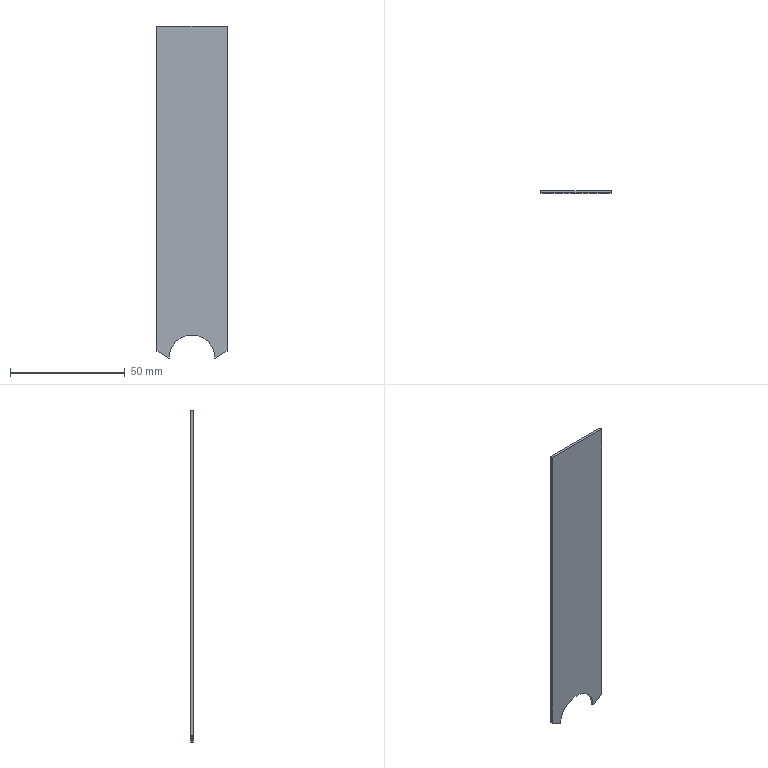Part | STEP file | solid 164 | 1 solid | 10 faces | box 30.5 x 1 x 144.425 mm | volume 4236 mm3 | plane 5 | cylinder 3 | cone 2 | commonest cylinder face diameters 30.5 x2 20 x1